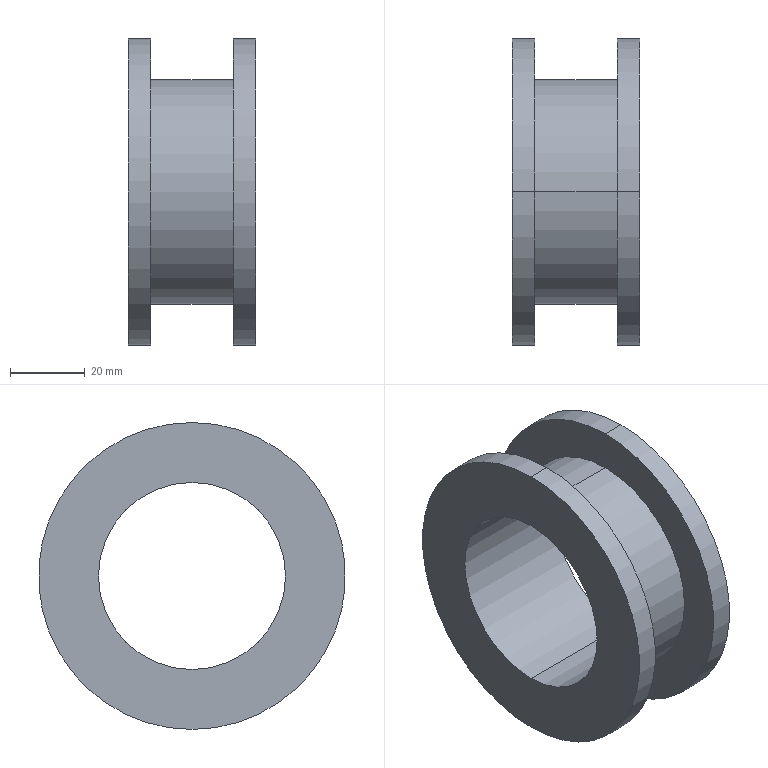Part | SolidWorks | features Revolution 1 | 1 solid | 12 faces | box 34 x 82 x 82 mm | volume 58817 mm3 | cylinder 8 | plane 4 | commonest cylinder face diameters 82 x4 50 x2 60 x2
STEP:
#1=CARTESIAN_POINT('',(34.,0.,-25.));
#2=VERTEX_POINT('',#1);
#3=CARTESIAN_POINT('',(34.,0.,25.));
#4=VERTEX_POINT('',#3);
#5=CARTESIAN_POINT('',(34.,0.,0.));
#6=DIRECTION('',(-1.,0.,0.));
#7=DIRECTION('',(0.,0.,1.));
#8=AXIS2_PLACEMENT_3D('',#5,#6,#7);
#9=CIRCLE('',#8,25.);
#10=EDGE_CURVE('',#2,#4,#9,.T.);
#11=ORIENTED_EDGE('',*,*,#10,.F.);
#12=CARTESIAN_POINT('',(0.,0.,-25.));
#13=VERTEX_POINT('',#12);
#14=CARTESIAN_POINT('',(0.,0.,-25.));
#15=DIRECTION('',(-1.,0.,0.));
#16=VECTOR('',#15,1000.);
#17=LINE('',#14,#16);
#18=EDGE_CURVE('',#2,#13,#17,.T.);
#19=ORIENTED_EDGE('',*,*,#18,.T.);
#20=CARTESIAN_POINT('',(0.,0.,25.));
#21=VERTEX_POINT('',#20);
#22=CARTESIAN_POINT('',(0.,0.,0.));
#23=DIRECTION('',(-1.,0.,0.));
#24=DIRECTION('',(0.,0.,1.));
#25=AXIS2_PLACEMENT_3D('',#22,#23,#24);
#26=CIRCLE('',#25,25.);
#27=EDGE_CURVE('',#13,#21,#26,.T.);
#28=ORIENTED_EDGE('',*,*,#27,.T.);
#29=CARTESIAN_POINT('',(0.,0.,25.));
#30=DIRECTION('',(-1.,0.,0.));
#31=VECTOR('',#30,1000.);
#32=LINE('',#29,#31);
#33=EDGE_CURVE('',#4,#21,#32,.T.);
#34=ORIENTED_EDGE('',*,*,#33,.F.);
#35=EDGE_LOOP('',(#11,#19,#28,#34));
#36=FACE_OUTER_BOUND('',#35,.T.);
#37=CARTESIAN_POINT('',(0.,0.,0.));
#38=DIRECTION('',(-1.,0.,0.));
#39=DIRECTION('',(0.,0.,1.));
#40=AXIS2_PLACEMENT_3D('',#37,#38,#39);
#41=CYLINDRICAL_SURFACE('',#40,25.);
#42=ADVANCED_FACE('',(#36),#41,.F.);
#43=CARTESIAN_POINT('',(34.,0.,41.));
#44=VERTEX_POINT('',#43);
#45=CARTESIAN_POINT('',(34.,0.,-41.));
#46=VERTEX_POINT('',#45);
#47=CARTESIAN_POINT('',(34.,0.,0.));
#48=DIRECTION('',(-1.,0.,0.));
#49=DIRECTION('',(0.,0.,1.));
#50=AXIS2_PLACEMENT_3D('',#47,#48,#49);
#51=CIRCLE('',#50,41.);
#52=EDGE_CURVE('',#44,#46,#51,.T.);
#53=ORIENTED_EDGE('',*,*,#52,.T.);
#54=CARTESIAN_POINT('',(28.,0.,-41.));
#55=VERTEX_POINT('',#54);
#56=CARTESIAN_POINT('',(0.,0.,-41.));
#57=DIRECTION('',(-1.,0.,0.));
#58=VECTOR('',#57,1000.);
#59=LINE('',#56,#58);
#60=EDGE_CURVE('',#46,#55,#59,.T.);
#61=ORIENTED_EDGE('',*,*,#60,.T.);
#62=CARTESIAN_POINT('',(28.,0.,41.));
#63=VERTEX_POINT('',#62);
#64=CARTESIAN_POINT('',(28.,0.,0.));
#65=DIRECTION('',(-1.,0.,0.));
#66=DIRECTION('',(0.,0.,1.));
#67=AXIS2_PLACEMENT_3D('',#64,#65,#66);
#68=CIRCLE('',#67,41.);
#69=EDGE_CURVE('',#63,#55,#68,.T.);
#70=ORIENTED_EDGE('',*,*,#69,.F.);
#71=CARTESIAN_POINT('',(0.,0.,41.));
#72=DIRECTION('',(-1.,0.,0.));
#73=VECTOR('',#72,1000.);
#74=LINE('',#71,#73);
#75=EDGE_CURVE('',#44,#63,#74,.T.);
#76=ORIENTED_EDGE('',*,*,#75,.F.);
#77=EDGE_LOOP('',(#53,#61,#70,#76));
#78=FACE_OUTER_BOUND('',#77,.T.);
#79=CARTESIAN_POINT('',(0.,0.,0.));
#80=DIRECTION('',(-1.,0.,0.));
#81=DIRECTION('',(0.,0.,1.));
#82=AXIS2_PLACEMENT_3D('',#79,#80,#81);
#83=CYLINDRICAL_SURFACE('',#82,41.);
#84=ADVANCED_FACE('',(#78),#83,.T.);
#85=CARTESIAN_POINT('',(28.,0.,30.));
#86=VERTEX_POINT('',#85);
#87=CARTESIAN_POINT('',(28.,0.,-30.));
#88=VERTEX_POINT('',#87);
#89=CARTESIAN_POINT('',(28.,0.,0.));
#90=DIRECTION('',(-1.,0.,0.));
#91=DIRECTION('',(0.,0.,1.));
#92=AXIS2_PLACEMENT_3D('',#89,#90,#91);
#93=CIRCLE('',#92,30.);
#94=EDGE_CURVE('',#86,#88,#93,.T.);
#95=ORIENTED_EDGE('',*,*,#94,.T.);
#96=CARTESIAN_POINT('',(6.,0.,-30.));
#97=VERTEX_POINT('',#96);
#98=CARTESIAN_POINT('',(0.,0.,-30.));
#99=DIRECTION('',(-1.,0.,0.));
#100=VECTOR('',#99,1000.);
#101=LINE('',#98,#100);
#102=EDGE_CURVE('',#88,#97,#101,.T.);
#103=ORIENTED_EDGE('',*,*,#102,.T.);
#104=CARTESIAN_POINT('',(6.,0.,30.));
#105=VERTEX_POINT('',#104);
#106=CARTESIAN_POINT('',(6.,0.,0.));
#107=DIRECTION('',(-1.,0.,0.));
#108=DIRECTION('',(0.,0.,1.));
#109=AXIS2_PLACEMENT_3D('',#106,#107,#108);
#110=CIRCLE('',#109,30.);
#111=EDGE_CURVE('',#105,#97,#110,.T.);
#112=ORIENTED_EDGE('',*,*,#111,.F.);
#113=CARTESIAN_POINT('',(0.,0.,30.));
#114=DIRECTION('',(-1.,0.,0.));
#115=VECTOR('',#114,1000.);
#116=LINE('',#113,#115);
#117=EDGE_CURVE('',#86,#105,#116,.T.);
#118=ORIENTED_EDGE('',*,*,#117,.F.);
#119=EDGE_LOOP('',(#95,#103,#112,#118));
#120=FACE_OUTER_BOUND('',#119,.T.);
#121=CARTESIAN_POINT('',(0.,0.,0.));
#122=DIRECTION('',(-1.,0.,0.));
#123=DIRECTION('',(0.,0.,1.));
#124=AXIS2_PLACEMENT_3D('',#121,#122,#123);
#125=CYLINDRICAL_SURFACE('',#124,30.);
#126=ADVANCED_FACE('',(#120),#125,.T.);
#127=CARTESIAN_POINT('',(6.,0.,41.));
#128=VERTEX_POINT('',#127);
#129=CARTESIAN_POINT('',(6.,0.,-41.));
#130=VERTEX_POINT('',#129);
#131=CARTESIAN_POINT('',(6.,0.,0.));
#132=DIRECTION('',(-1.,0.,0.));
#133=DIRECTION('',(0.,0.,1.));
#134=AXIS2_PLACEMENT_3D('',#131,#132,#133);
#135=CIRCLE('',#134,41.);
#136=EDGE_CURVE('',#128,#130,#135,.T.);
#137=ORIENTED_EDGE('',*,*,#136,.T.);
#138=CARTESIAN_POINT('',(0.,0.,-41.));
#139=VERTEX_POINT('',#138);
#140=CARTESIAN_POINT('',(0.,0.,-41.));
#141=DIRECTION('',(-1.,0.,0.));
#142=VECTOR('',#141,1000.);
#143=LINE('',#140,#142);
#144=EDGE_CURVE('',#130,#139,#143,.T.);
#145=ORIENTED_EDGE('',*,*,#144,.T.);
#146=CARTESIAN_POINT('',(0.,0.,41.));
#147=VERTEX_POINT('',#146);
#148=CARTESIAN_POINT('',(0.,0.,0.));
#149=DIRECTION('',(-1.,0.,0.));
#150=DIRECTION('',(0.,0.,1.));
#151=AXIS2_PLACEMENT_3D('',#148,#149,#150);
#152=CIRCLE('',#151,41.);
#153=EDGE_CURVE('',#147,#139,#152,.T.);
#154=ORIENTED_EDGE('',*,*,#153,.F.);
#155=CARTESIAN_POINT('',(0.,0.,41.));
#156=DIRECTION('',(-1.,0.,0.));
#157=VECTOR('',#156,1000.);
#158=LINE('',#155,#157);
#159=EDGE_CURVE('',#128,#147,#158,.T.);
#160=ORIENTED_EDGE('',*,*,#159,.F.);
#161=EDGE_LOOP('',(#137,#145,#154,#160));
#162=FACE_OUTER_BOUND('',#161,.T.);
#163=CARTESIAN_POINT('',(0.,0.,0.));
#164=DIRECTION('',(-1.,0.,0.));
#165=DIRECTION('',(0.,0.,1.));
#166=AXIS2_PLACEMENT_3D('',#163,#164,#165);
#167=CYLINDRICAL_SURFACE('',#166,41.);
#168=ADVANCED_FACE('',(#162),#167,.T.);
#169=ORIENTED_EDGE('',*,*,#144,.F.);
#170=CARTESIAN_POINT('',(6.,0.,0.));
#171=DIRECTION('',(-1.,0.,0.));
#172=DIRECTION('',(0.,0.,1.));
#173=AXIS2_PLACEMENT_3D('',#170,#171,#172);
#174=CIRCLE('',#173,41.);
#175=EDGE_CURVE('',#130,#128,#174,.T.);
#176=ORIENTED_EDGE('',*,*,#175,.T.);
#177=ORIENTED_EDGE('',*,*,#159,.T.);
#178=CARTESIAN_POINT('',(0.,0.,0.));
#179=DIRECTION('',(-1.,0.,0.));
#180=DIRECTION('',(0.,0.,1.));
#181=AXIS2_PLACEMENT_3D('',#178,#179,#180);
#182=CIRCLE('',#181,41.);
#183=EDGE_CURVE('',#139,#147,#182,.T.);
#184=ORIENTED_EDGE('',*,*,#183,.F.);
#185=EDGE_LOOP('',(#169,#176,#177,#184));
#186=FACE_OUTER_BOUND('',#185,.T.);
#187=CARTESIAN_POINT('',(0.,0.,0.));
#188=DIRECTION('',(-1.,0.,0.));
#189=DIRECTION('',(0.,0.,1.));
#190=AXIS2_PLACEMENT_3D('',#187,#188,#189);
#191=CYLINDRICAL_SURFACE('',#190,41.);
#192=ADVANCED_FACE('',(#186),#191,.T.);
#193=ORIENTED_EDGE('',*,*,#136,.F.);
#194=ORIENTED_EDGE('',*,*,#175,.F.);
#195=EDGE_LOOP('',(#193,#194));
#196=FACE_OUTER_BOUND('',#195,.T.);
#197=ORIENTED_EDGE('',*,*,#111,.T.);
#198=CARTESIAN_POINT('',(6.,0.,0.));
#199=DIRECTION('',(-1.,0.,0.));
#200=DIRECTION('',(0.,0.,1.));
#201=AXIS2_PLACEMENT_3D('',#198,#199,#200);
#202=CIRCLE('',#201,30.);
#203=EDGE_CURVE('',#97,#105,#202,.T.);
#204=ORIENTED_EDGE('',*,*,#203,.T.);
#205=EDGE_LOOP('',(#197,#204));
#206=FACE_BOUND('',#205,.T.);
#207=CARTESIAN_POINT('',(6.,41.,0.));
#208=DIRECTION('',(-1.,0.,0.));
#209=DIRECTION('',(0.,0.,1.));
#210=AXIS2_PLACEMENT_3D('',#207,#208,#209);
#211=PLANE('',#210);
#212=ADVANCED_FACE('',(#196,#206),#211,.F.);
#213=ORIENTED_EDGE('',*,*,#102,.F.);
#214=CARTESIAN_POINT('',(28.,0.,0.));
#215=DIRECTION('',(-1.,0.,0.));
#216=DIRECTION('',(0.,0.,1.));
#217=AXIS2_PLACEMENT_3D('',#214,#215,#216);
#218=CIRCLE('',#217,30.);
#219=EDGE_CURVE('',#88,#86,#218,.T.);
#220=ORIENTED_EDGE('',*,*,#219,.T.);
#221=ORIENTED_EDGE('',*,*,#117,.T.);
#222=ORIENTED_EDGE('',*,*,#203,.F.);
#223=EDGE_LOOP('',(#213,#220,#221,#222));
#224=FACE_OUTER_BOUND('',#223,.T.);
#225=CARTESIAN_POINT('',(0.,0.,0.));
#226=DIRECTION('',(-1.,0.,0.));
#227=DIRECTION('',(0.,0.,1.));
#228=AXIS2_PLACEMENT_3D('',#225,#226,#227);
#229=CYLINDRICAL_SURFACE('',#228,30.);
#230=ADVANCED_FACE('',(#224),#229,.T.);
#231=ORIENTED_EDGE('',*,*,#94,.F.);
#232=ORIENTED_EDGE('',*,*,#219,.F.);
#233=EDGE_LOOP('',(#231,#232));
#234=FACE_BOUND('',#233,.T.);
#235=ORIENTED_EDGE('',*,*,#69,.T.);
#236=CARTESIAN_POINT('',(28.,0.,0.));
#237=DIRECTION('',(-1.,0.,0.));
#238=DIRECTION('',(0.,0.,1.));
#239=AXIS2_PLACEMENT_3D('',#236,#237,#238);
#240=CIRCLE('',#239,41.);
#241=EDGE_CURVE('',#55,#63,#240,.T.);
#242=ORIENTED_EDGE('',*,*,#241,.T.);
#243=EDGE_LOOP('',(#235,#242));
#244=FACE_OUTER_BOUND('',#243,.T.);
#245=CARTESIAN_POINT('',(28.,30.,0.));
#246=DIRECTION('',(1.,0.,0.));
#247=DIRECTION('',(0.,0.,-1.));
#248=AXIS2_PLACEMENT_3D('',#245,#246,#247);
#249=PLANE('',#248);
#250=ADVANCED_FACE('',(#234,#244),#249,.F.);
#251=ORIENTED_EDGE('',*,*,#60,.F.);
#252=CARTESIAN_POINT('',(34.,0.,0.));
#253=DIRECTION('',(-1.,0.,0.));
#254=DIRECTION('',(0.,0.,1.));
#255=AXIS2_PLACEMENT_3D('',#252,#253,#254);
#256=CIRCLE('',#255,41.);
#257=EDGE_CURVE('',#46,#44,#256,.T.);
#258=ORIENTED_EDGE('',*,*,#257,.T.);
#259=ORIENTED_EDGE('',*,*,#75,.T.);
#260=ORIENTED_EDGE('',*,*,#241,.F.);
#261=EDGE_LOOP('',(#251,#258,#259,#260));
#262=FACE_OUTER_BOUND('',#261,.T.);
#263=CARTESIAN_POINT('',(0.,0.,0.));
#264=DIRECTION('',(-1.,0.,0.));
#265=DIRECTION('',(0.,0.,1.));
#266=AXIS2_PLACEMENT_3D('',#263,#264,#265);
#267=CYLINDRICAL_SURFACE('',#266,41.);
#268=ADVANCED_FACE('',(#262),#267,.T.);
#269=ORIENTED_EDGE('',*,*,#52,.F.);
#270=ORIENTED_EDGE('',*,*,#257,.F.);
#271=EDGE_LOOP('',(#269,#270));
#272=FACE_OUTER_BOUND('',#271,.T.);
#273=CARTESIAN_POINT('',(34.,0.,0.));
#274=DIRECTION('',(-1.,0.,0.));
#275=DIRECTION('',(0.,0.,1.));
#276=AXIS2_PLACEMENT_3D('',#273,#274,#275);
#277=CIRCLE('',#276,25.);
#278=EDGE_CURVE('',#4,#2,#277,.T.);
#279=ORIENTED_EDGE('',*,*,#278,.T.);
#280=ORIENTED_EDGE('',*,*,#10,.T.);
#281=EDGE_LOOP('',(#279,#280));
#282=FACE_BOUND('',#281,.T.);
#283=CARTESIAN_POINT('',(34.,41.,0.));
#284=DIRECTION('',(-1.,0.,0.));
#285=DIRECTION('',(0.,0.,1.));
#286=AXIS2_PLACEMENT_3D('',#283,#284,#285);
#287=PLANE('',#286);
#288=ADVANCED_FACE('',(#272,#282),#287,.F.);
#289=ORIENTED_EDGE('',*,*,#18,.F.);
#290=ORIENTED_EDGE('',*,*,#278,.F.);
#291=ORIENTED_EDGE('',*,*,#33,.T.);
#292=CARTESIAN_POINT('',(0.,0.,0.));
#293=DIRECTION('',(-1.,0.,0.));
#294=DIRECTION('',(0.,0.,1.));
#295=AXIS2_PLACEMENT_3D('',#292,#293,#294);
#296=CIRCLE('',#295,25.);
#297=EDGE_CURVE('',#21,#13,#296,.T.);
#298=ORIENTED_EDGE('',*,*,#297,.T.);
#299=EDGE_LOOP('',(#289,#290,#291,#298));
#300=FACE_OUTER_BOUND('',#299,.T.);
#301=CARTESIAN_POINT('',(0.,0.,0.));
#302=DIRECTION('',(-1.,0.,0.));
#303=DIRECTION('',(0.,0.,1.));
#304=AXIS2_PLACEMENT_3D('',#301,#302,#303);
#305=CYLINDRICAL_SURFACE('',#304,25.);
#306=ADVANCED_FACE('',(#300),#305,.F.);
#307=ORIENTED_EDGE('',*,*,#297,.F.);
#308=ORIENTED_EDGE('',*,*,#27,.F.);
#309=EDGE_LOOP('',(#307,#308));
#310=FACE_BOUND('',#309,.T.);
#311=ORIENTED_EDGE('',*,*,#153,.T.);
#312=ORIENTED_EDGE('',*,*,#183,.T.);
#313=EDGE_LOOP('',(#311,#312));
#314=FACE_OUTER_BOUND('',#313,.T.);
#315=CARTESIAN_POINT('',(0.,25.,0.));
#316=DIRECTION('',(1.,0.,0.));
#317=DIRECTION('',(0.,0.,-1.));
#318=AXIS2_PLACEMENT_3D('',#315,#316,#317);
#319=PLANE('',#318);
#320=ADVANCED_FACE('',(#310,#314),#319,.F.);
#321=CLOSED_SHELL('',(#42,#84,#126,#168,#192,#212,#230,#250,#268,#288,#306,#320));
#322=MANIFOLD_SOLID_BREP('',#321);
#323=CARTESIAN_POINT('',(0.,0.,0.));
#324=DIRECTION('',(0.,0.,1.));
#325=DIRECTION('',(1.,0.,0.));
#326=AXIS2_PLACEMENT_3D('',#323,#324,#325);
#327=(LENGTH_UNIT()NAMED_UNIT(*)SI_UNIT(.MILLI.,.METRE.));
#328=UNCERTAINTY_MEASURE_WITH_UNIT(LENGTH_MEASURE(0.00001),#327,'','');
#329=(NAMED_UNIT(*)PLANE_ANGLE_UNIT()SI_UNIT($,.RADIAN.));
#330=(NAMED_UNIT(*)SI_UNIT($,.STERADIAN.)SOLID_ANGLE_UNIT());
#331=(GEOMETRIC_REPRESENTATION_CONTEXT(3)GLOBAL_UNCERTAINTY_ASSIGNED_CONTEXT((#328))GLOBAL_UNIT_ASSIGNED_CONTEXT((#327,#329,#330))REPRESENTATION_CONTEXT('',''));
#332=ADVANCED_BREP_SHAPE_REPRESENTATION('',(#322,#326),#331);